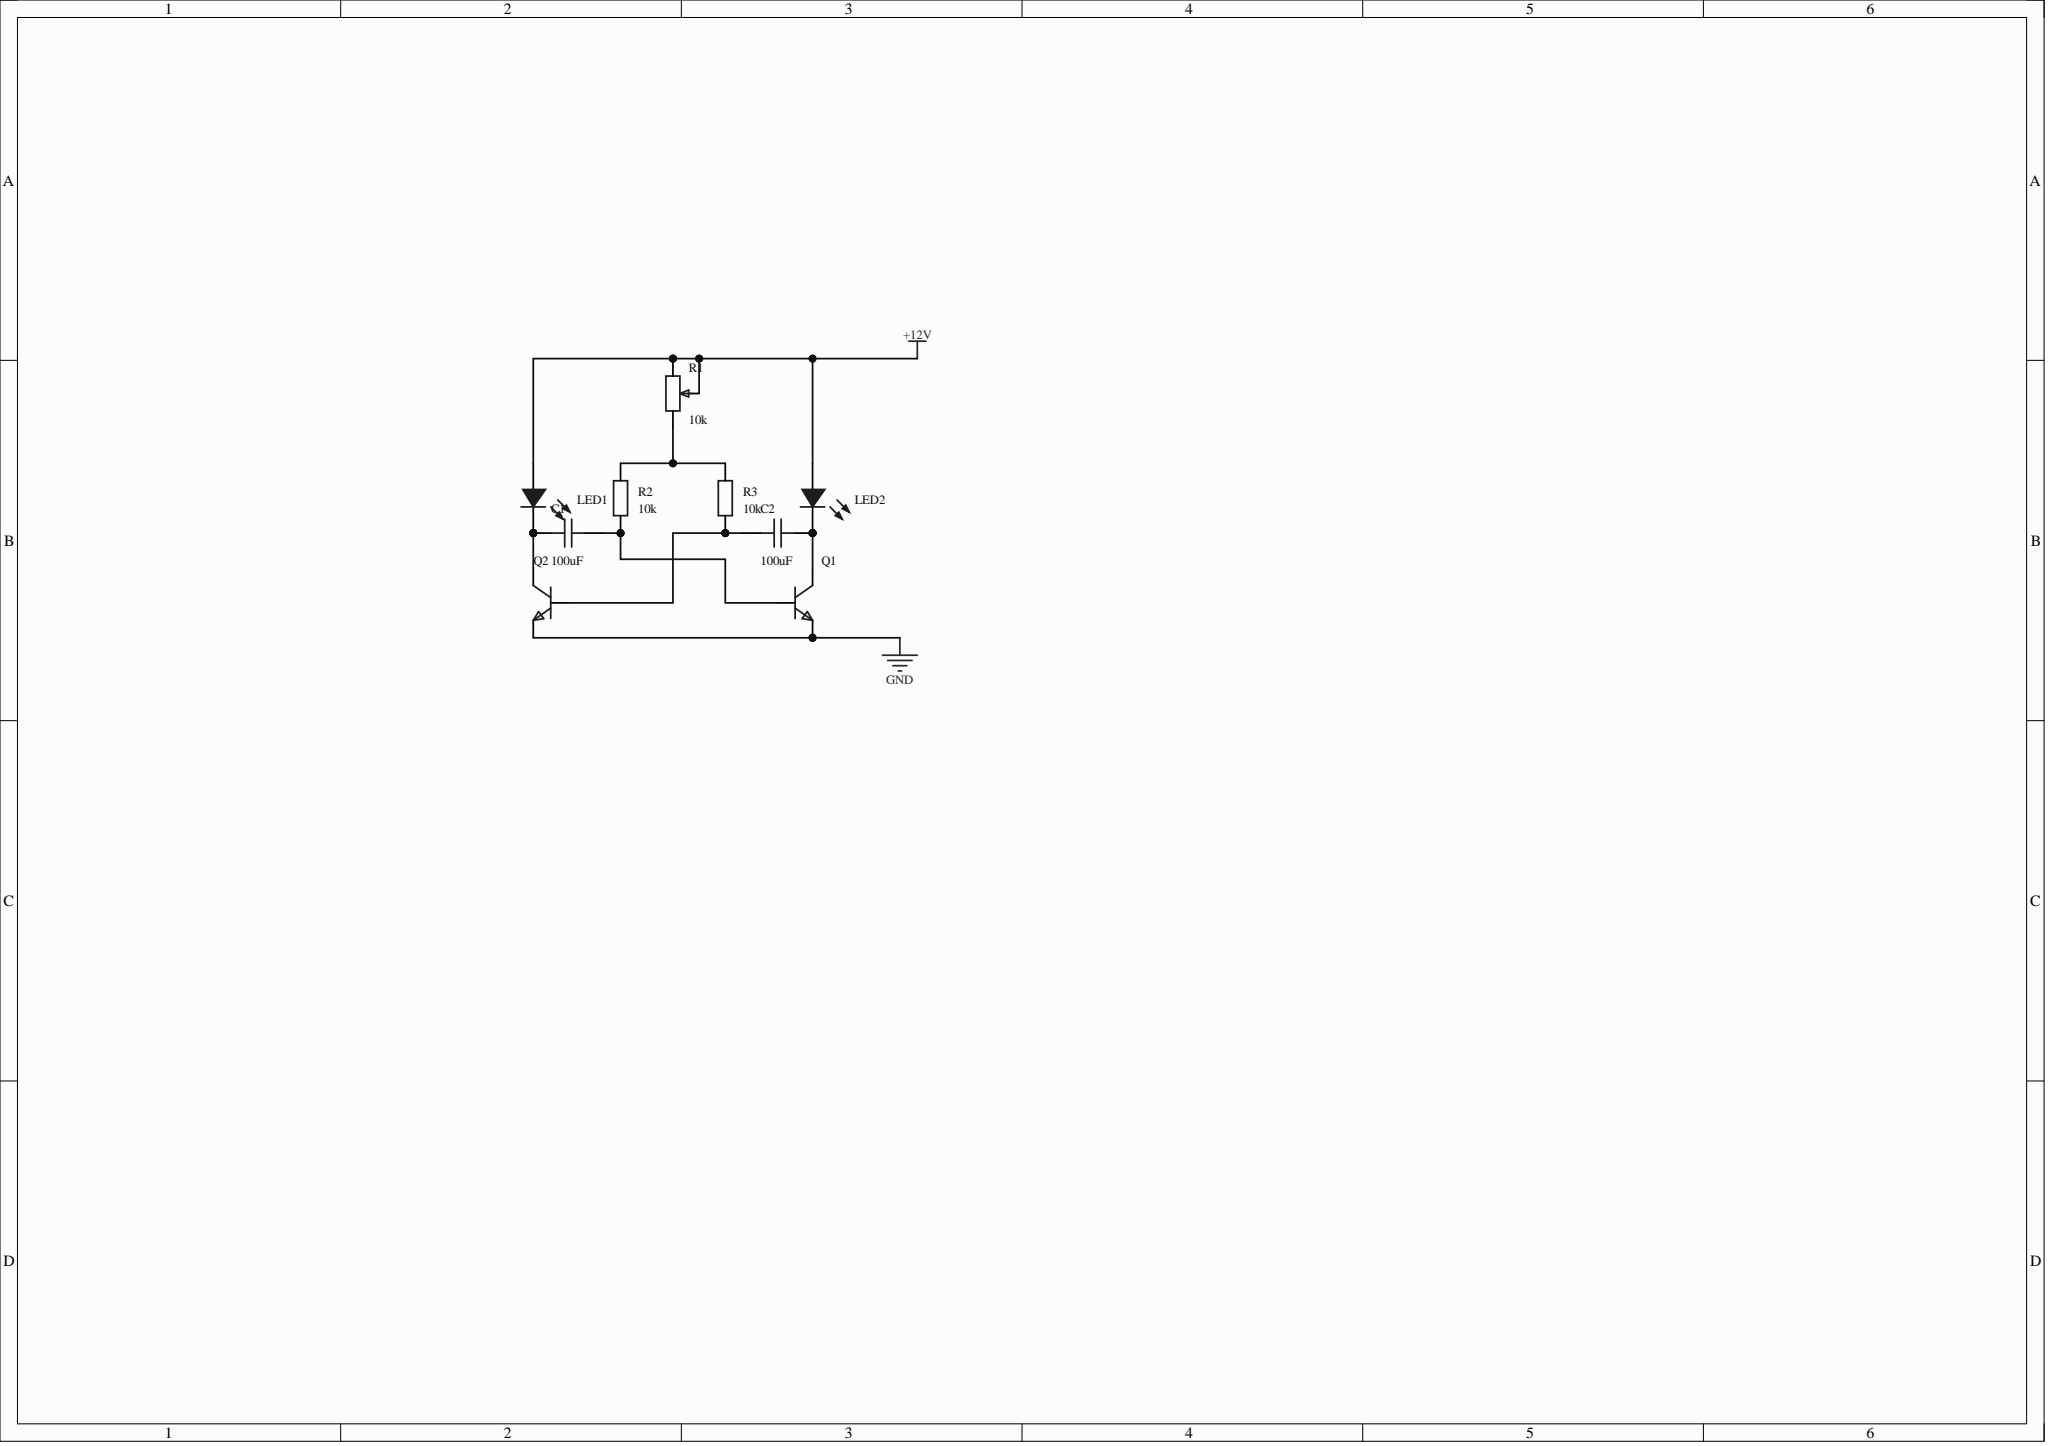Circuit board | Altium Designer | 9 parts | 7 nets
Bill of materials:
Comment,Description,Designator,Footprint,LibRef,Quantity
"100uF","容值:100nF;精度:±10%;额定电压:50V;温度系数:X7R;","C1, C2","CAP-TH_L5.1-W3.2-P5.08-D0.50","C323C104K5R5TA7301","2"
"","","LED1, LED2","LED_TH-3mm","LED_TH-B_3mm","2"
"","","Q1, Q2","S8050_TO_92","S8050_TO_NPN","2"
"10k","","R1","R_3296","R_3296","1"
"10k","","R2, R3","Res_1/8W","Res_AXIAL-1/8W","2"
Netlist (Protel format):
[
C1
CAP-TH_L5.1-W3.2-P5.08-D0.50
100uF



]
[
C2
CAP-TH_L5.1-W3.2-P5.08-D0.50
100uF



]
[
LED1
LED_TH-3mm




]
[
LED2
LED_TH-3mm




]
[
Q1
S8050_TO_92




]
[
Q2
S8050_TO_92




]
[
R1
R_3296
10k



]
[
R2
Res_1/8W
10k



]
[
R3
Res_1/8W
10k



]
(
NetR1_1
R1-1
R2-2
R3-2
)
(
NetC2_2
C2-2
Q2-2
R3-1
)
(
NetC2_1
C2-1
LED2-2
Q1-3
)
(
NetC1_2
C1-2
Q1-2
R2-1
)
(
NetC1_1
C1-1
LED1-2
Q2-3
)
(
GND
Q1-1
Q2-1
)
(
+12V
LED1-1
LED2-1
R1-2
R1-3
)